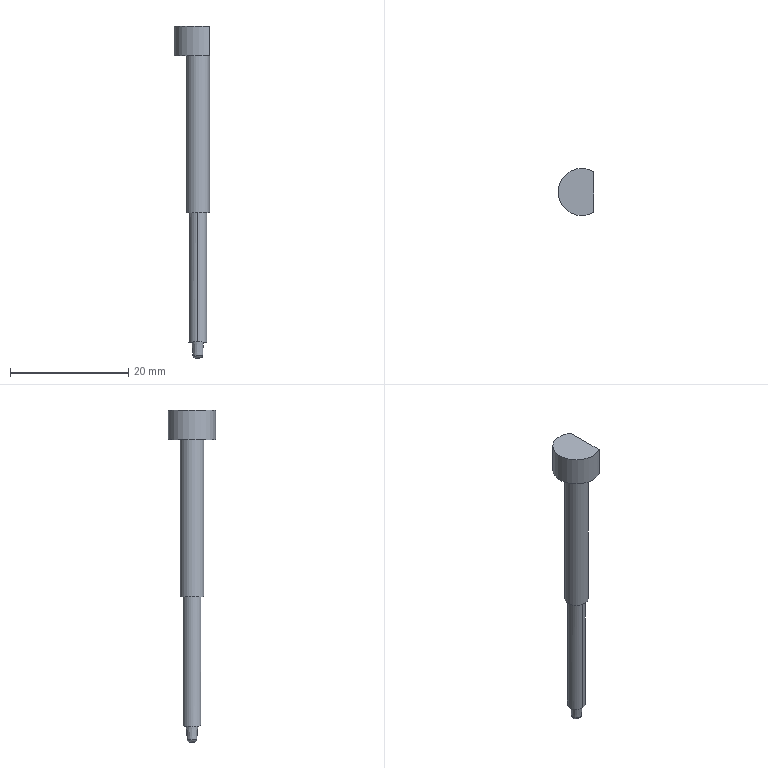Part | NX | features solid 2 | 1 solid | 12 faces | box 6 x 8 x 56.264 mm | volume 699.912 mm3 | plane 5 | cylinder 4 | cone 2 | torus 1 | commonest cylinder face diameters 3.015 x2 4 x1 8 x1
STEP:
#1=CARTESIAN_POINT('',(2.,-37.688,38.875));
#2=VERTEX_POINT('',#1);
#3=CARTESIAN_POINT('',(0.,-37.688,38.875));
#4=DIRECTION('',(0.,0.,1.));
#5=DIRECTION('',(1.,0.,0.));
#6=AXIS2_PLACEMENT_3D('',#3,#4,#5);
#7=CIRCLE('',#6,2.);
#8=EDGE_CURVE('',#2,#2,#7,.F.);
#9=ORIENTED_EDGE('',*,*,#8,.F.);
#10=EDGE_LOOP('',(#9));
#11=FACE_BOUND('',#10,.T.);
#12=CARTESIAN_POINT('',(2.,-37.688,65.5));
#13=VERTEX_POINT('',#12);
#14=CARTESIAN_POINT('',(0.,-37.688,65.5));
#15=DIRECTION('',(0.,0.,-1.));
#16=DIRECTION('',(-1.,0.,0.));
#17=AXIS2_PLACEMENT_3D('',#14,#15,#16);
#18=CIRCLE('',#17,2.);
#19=EDGE_CURVE('',#13,#13,#18,.F.);
#20=ORIENTED_EDGE('',*,*,#19,.F.);
#21=EDGE_LOOP('',(#20));
#22=FACE_BOUND('',#21,.T.);
#23=CARTESIAN_POINT('',(0.,-37.688,117.875));
#24=DIRECTION('',(0.,0.,-1.));
#25=DIRECTION('',(-1.,0.,0.));
#26=AXIS2_PLACEMENT_3D('',#23,#24,#25);
#27=CYLINDRICAL_SURFACE('',#26,2.);
#28=ADVANCED_FACE('',(#11,#22),#27,.T.);
#29=CARTESIAN_POINT('',(2.,-41.152,65.5));
#30=VERTEX_POINT('',#29);
#31=CARTESIAN_POINT('',(2.,-34.223,65.5));
#32=VERTEX_POINT('',#31);
#33=CARTESIAN_POINT('',(0.,-37.688,65.5));
#34=DIRECTION('',(0.,0.,-1.));
#35=DIRECTION('',(-1.,0.,0.));
#36=AXIS2_PLACEMENT_3D('',#33,#34,#35);
#37=CIRCLE('',#36,4.);
#38=EDGE_CURVE('',#30,#32,#37,.T.);
#39=ORIENTED_EDGE('',*,*,#38,.F.);
#40=CARTESIAN_POINT('',(2.,-41.152,70.5));
#41=VERTEX_POINT('',#40);
#42=CARTESIAN_POINT('',(2.,-41.152,66.5));
#43=DIRECTION('',(0.,0.,1.));
#44=VECTOR('',#43,1000.);
#45=LINE('',#42,#44);
#46=EDGE_CURVE('',#41,#30,#45,.F.);
#47=ORIENTED_EDGE('',*,*,#46,.F.);
#48=CARTESIAN_POINT('',(2.,-34.223,70.5));
#49=VERTEX_POINT('',#48);
#50=CARTESIAN_POINT('',(0.,-37.688,70.5));
#51=DIRECTION('',(0.,0.,1.));
#52=DIRECTION('',(1.,0.,0.));
#53=AXIS2_PLACEMENT_3D('',#50,#51,#52);
#54=CIRCLE('',#53,4.);
#55=EDGE_CURVE('',#41,#49,#54,.F.);
#56=ORIENTED_EDGE('',*,*,#55,.T.);
#57=CARTESIAN_POINT('',(2.,-34.223,66.5));
#58=DIRECTION('',(0.,0.,1.));
#59=VECTOR('',#58,1000.);
#60=LINE('',#57,#59);
#61=EDGE_CURVE('',#32,#49,#60,.T.);
#62=ORIENTED_EDGE('',*,*,#61,.F.);
#63=EDGE_LOOP('',(#39,#47,#56,#62));
#64=FACE_BOUND('',#63,.T.);
#65=CARTESIAN_POINT('',(0.,-37.688,66.5));
#66=DIRECTION('',(0.,0.,1.));
#67=DIRECTION('',(1.,0.,0.));
#68=AXIS2_PLACEMENT_3D('',#65,#66,#67);
#69=CYLINDRICAL_SURFACE('',#68,4.);
#70=ADVANCED_FACE('',(#64),#69,.T.);
#71=CARTESIAN_POINT('',(2.,37.688,65.5));
#72=DIRECTION('',(0.,-1.,0.));
#73=VECTOR('',#72,1000.);
#74=LINE('',#71,#73);
#75=EDGE_CURVE('',#13,#32,#74,.F.);
#76=ORIENTED_EDGE('',*,*,#75,.F.);
#77=ORIENTED_EDGE('',*,*,#19,.T.);
#78=CARTESIAN_POINT('',(2.,37.688,65.5));
#79=DIRECTION('',(0.,-1.,0.));
#80=VECTOR('',#79,1000.);
#81=LINE('',#78,#80);
#82=EDGE_CURVE('',#30,#13,#81,.F.);
#83=ORIENTED_EDGE('',*,*,#82,.F.);
#84=ORIENTED_EDGE('',*,*,#38,.T.);
#85=EDGE_LOOP('',(#76,#77,#83,#84));
#86=FACE_BOUND('',#85,.T.);
#87=CARTESIAN_POINT('',(0.,37.688,65.5));
#88=DIRECTION('',(0.,0.,-1.));
#89=DIRECTION('',(-1.,0.,0.));
#90=AXIS2_PLACEMENT_3D('',#87,#88,#89);
#91=PLANE('',#90);
#92=ADVANCED_FACE('',(#86),#91,.T.);
#93=CARTESIAN_POINT('',(2.,0.,70.5));
#94=DIRECTION('',(0.,1.,0.));
#95=VECTOR('',#94,1000.);
#96=LINE('',#93,#95);
#97=EDGE_CURVE('',#49,#41,#96,.F.);
#98=ORIENTED_EDGE('',*,*,#97,.F.);
#99=ORIENTED_EDGE('',*,*,#55,.F.);
#100=EDGE_LOOP('',(#98,#99));
#101=FACE_BOUND('',#100,.T.);
#102=CARTESIAN_POINT('',(0.,0.,70.5));
#103=DIRECTION('',(0.,0.,1.));
#104=DIRECTION('',(1.,0.,0.));
#105=AXIS2_PLACEMENT_3D('',#102,#103,#104);
#106=PLANE('',#105);
#107=ADVANCED_FACE('',(#101),#106,.T.);
#108=CARTESIAN_POINT('',(0.,-36.18,38.875));
#109=VERTEX_POINT('',#108);
#110=CARTESIAN_POINT('',(0.,-39.195,38.875));
#111=VERTEX_POINT('',#110);
#112=CARTESIAN_POINT('',(0.,-37.688,38.875));
#113=DIRECTION('',(0.,0.,1.));
#114=DIRECTION('',(0.,-1.,0.));
#115=AXIS2_PLACEMENT_3D('',#112,#113,#114);
#116=CIRCLE('',#115,1.508);
#117=EDGE_CURVE('',#109,#111,#116,.F.);
#118=ORIENTED_EDGE('',*,*,#117,.T.);
#119=CARTESIAN_POINT('',(0.,-39.195,16.996));
#120=VERTEX_POINT('',#119);
#121=CARTESIAN_POINT('',(0.,-39.195,38.875));
#122=DIRECTION('',(0.,0.,-1.));
#123=VECTOR('',#122,1000.);
#124=LINE('',#121,#123);
#125=EDGE_CURVE('',#120,#111,#124,.F.);
#126=ORIENTED_EDGE('',*,*,#125,.F.);
#127=CARTESIAN_POINT('',(0.,-36.18,16.969));
#128=VERTEX_POINT('',#127);
#129=CARTESIAN_POINT('',(0.,-39.195,16.996));
#130=CARTESIAN_POINT('',(0.3992,-39.195,16.996));
#131=CARTESIAN_POINT('',(1.178,-38.868,16.924));
#132=CARTESIAN_POINT('',(1.672,-37.691,16.809));
#133=CARTESIAN_POINT('',(1.18,-36.507,16.903));
#134=CARTESIAN_POINT('',(0.3992,-36.18,16.969));
#135=CARTESIAN_POINT('',(0.,-36.18,16.969));
#136=B_SPLINE_CURVE_WITH_KNOTS('',3,(#129,#130,#131,#132,#133,#134,#135),.UNSPECIFIED.,.F.,.F.,(4,1,1,1,4),(0.,0.00118,0.002361,0.003541,0.004722),.UNSPECIFIED.);
#137=EDGE_CURVE('',#120,#128,#136,.T.);
#138=ORIENTED_EDGE('',*,*,#137,.T.);
#139=CARTESIAN_POINT('',(0.,-36.18,16.969));
#140=DIRECTION('',(0.,0.,1.));
#141=VECTOR('',#140,1000.);
#142=LINE('',#139,#141);
#143=EDGE_CURVE('',#109,#128,#142,.F.);
#144=ORIENTED_EDGE('',*,*,#143,.F.);
#145=EDGE_LOOP('',(#118,#126,#138,#144));
#146=FACE_BOUND('',#145,.T.);
#147=CARTESIAN_POINT('',(0.,-37.688,38.875));
#148=DIRECTION('',(0.,0.,1.));
#149=DIRECTION('',(0.,1.,0.));
#150=AXIS2_PLACEMENT_3D('',#147,#148,#149);
#151=CYLINDRICAL_SURFACE('',#150,1.508);
#152=ADVANCED_FACE('',(#146),#151,.T.);
#153=CARTESIAN_POINT('',(0.,-37.688,38.875));
#154=DIRECTION('',(0.,0.,1.));
#155=DIRECTION('',(0.,1.,0.));
#156=AXIS2_PLACEMENT_3D('',#153,#154,#155);
#157=CIRCLE('',#156,1.508);
#158=EDGE_CURVE('',#111,#109,#157,.F.);
#159=ORIENTED_EDGE('',*,*,#158,.T.);
#160=ORIENTED_EDGE('',*,*,#143,.T.);
#161=CARTESIAN_POINT('',(0.,-36.18,16.969));
#162=CARTESIAN_POINT('',(-0.3992,-36.18,16.969));
#163=CARTESIAN_POINT('',(-1.179,-36.507,16.903));
#164=CARTESIAN_POINT('',(-1.672,-37.687,16.809));
#165=CARTESIAN_POINT('',(-1.179,-38.868,16.924));
#166=CARTESIAN_POINT('',(-0.3992,-39.195,16.996));
#167=CARTESIAN_POINT('',(0.,-39.195,16.996));
#168=B_SPLINE_CURVE_WITH_KNOTS('',3,(#161,#162,#163,#164,#165,#166,#167),.UNSPECIFIED.,.F.,.F.,(4,1,1,1,4),(0.,0.00118,0.002361,0.003541,0.004722),.UNSPECIFIED.);
#169=EDGE_CURVE('',#128,#120,#168,.T.);
#170=ORIENTED_EDGE('',*,*,#169,.T.);
#171=ORIENTED_EDGE('',*,*,#125,.T.);
#172=EDGE_LOOP('',(#159,#160,#170,#171));
#173=FACE_BOUND('',#172,.T.);
#174=CARTESIAN_POINT('',(0.,-37.688,38.875));
#175=DIRECTION('',(0.,0.,1.));
#176=DIRECTION('',(0.,1.,0.));
#177=AXIS2_PLACEMENT_3D('',#174,#175,#176);
#178=CYLINDRICAL_SURFACE('',#177,1.508);
#179=ADVANCED_FACE('',(#173),#178,.T.);
#180=ORIENTED_EDGE('',*,*,#8,.T.);
#181=EDGE_LOOP('',(#180));
#182=FACE_BOUND('',#181,.T.);
#183=ORIENTED_EDGE('',*,*,#158,.F.);
#184=ORIENTED_EDGE('',*,*,#117,.F.);
#185=EDGE_LOOP('',(#183,#184));
#186=FACE_BOUND('',#185,.T.);
#187=CARTESIAN_POINT('',(0.,-37.688,38.875));
#188=DIRECTION('',(0.,0.,1.));
#189=DIRECTION('',(0.,1.,0.));
#190=AXIS2_PLACEMENT_3D('',#187,#188,#189);
#191=PLANE('',#190);
#192=ADVANCED_FACE('',(#182,#186),#191,.F.);
#193=CARTESIAN_POINT('',(-0.3458,-37.688,14.236));
#194=VERTEX_POINT('',#193);
#195=CARTESIAN_POINT('',(0.,-37.688,14.236));
#196=DIRECTION('',(0.,0.,-1.));
#197=DIRECTION('',(-1.,0.,0.));
#198=AXIS2_PLACEMENT_3D('',#195,#196,#197);
#199=CIRCLE('',#198,0.3458);
#200=EDGE_CURVE('',#194,#194,#199,.T.);
#201=ORIENTED_EDGE('',*,*,#200,.T.);
#202=EDGE_LOOP('',(#201));
#203=FACE_BOUND('',#202,.T.);
#204=CARTESIAN_POINT('',(0.,-37.688,14.236));
#205=DIRECTION('',(0.,0.,-1.));
#206=DIRECTION('',(-1.,0.,0.));
#207=AXIS2_PLACEMENT_3D('',#204,#205,#206);
#208=PLANE('',#207);
#209=ADVANCED_FACE('',(#203),#208,.T.);
#210=CARTESIAN_POINT('',(-0.8451,-37.688,14.71));
#211=VERTEX_POINT('',#210);
#212=CARTESIAN_POINT('',(0.,-37.688,14.71));
#213=DIRECTION('',(0.,0.,-1.));
#214=DIRECTION('',(-1.,0.,0.));
#215=AXIS2_PLACEMENT_3D('',#212,#213,#214);
#216=CIRCLE('',#215,0.8451);
#217=EDGE_CURVE('',#211,#211,#216,.F.);
#218=ORIENTED_EDGE('',*,*,#217,.T.);
#219=EDGE_LOOP('',(#218));
#220=FACE_BOUND('',#219,.T.);
#221=CARTESIAN_POINT('',(0.8766,-37.292,16.933));
#222=VERTEX_POINT('',#221);
#223=CARTESIAN_POINT('',(0.3775,-36.688,16.977));
#224=CARTESIAN_POINT('',(0.9717,-37.25,16.923));
#225=CARTESIAN_POINT('',(0.9956,-38.066,16.926));
#226=CARTESIAN_POINT('',(0.4399,-38.661,16.991));
#227=CARTESIAN_POINT('',(-0.3781,-38.687,16.995));
#228=CARTESIAN_POINT('',(-0.9707,-38.127,16.931));
#229=CARTESIAN_POINT('',(-0.9966,-37.312,16.92));
#230=CARTESIAN_POINT('',(-0.4401,-36.714,16.974));
#231=CARTESIAN_POINT('',(0.3775,-36.688,16.977));
#232=CARTESIAN_POINT('',(0.9717,-37.25,16.923));
#233=CARTESIAN_POINT('',(0.9956,-38.066,16.926));
#234=B_SPLINE_CURVE_WITH_KNOTS('',3,(#223,#224,#225,#226,#227,#228,#229,#230,#231,#232,#233),.UNSPECIFIED.,.T.,.F.,(1,1,1,1,1,1,1,1,1,1,1,1,1,1,1),(-0.002259,-0.001506,-0.0007531,0.,0.0007531,0.001506,0.002259,0.003012,0.003765,0.004518,0.005272,0.006025,0.006778,0.007531,0.008284),.UNSPECIFIED.);
#235=EDGE_CURVE('',#222,#222,#234,.T.);
#236=ORIENTED_EDGE('',*,*,#235,.T.);
#237=EDGE_LOOP('',(#236));
#238=FACE_BOUND('',#237,.T.);
#239=CARTESIAN_POINT('',(0.,-37.688,14.236));
#240=DIRECTION('',(0.,0.,1.));
#241=DIRECTION('',(-1.,0.,0.));
#242=AXIS2_PLACEMENT_3D('',#239,#240,#241);
#243=CONICAL_SURFACE('',#242,0.8203,0.05236);
#244=ADVANCED_FACE('',(#220,#238),#243,.T.);
#245=ORIENTED_EDGE('',*,*,#235,.F.);
#246=EDGE_LOOP('',(#245));
#247=FACE_BOUND('',#246,.T.);
#248=ORIENTED_EDGE('',*,*,#137,.F.);
#249=ORIENTED_EDGE('',*,*,#169,.F.);
#250=EDGE_LOOP('',(#248,#249));
#251=FACE_BOUND('',#250,.T.);
#252=CARTESIAN_POINT('',(0.,-42.901,8.725));
#253=DIRECTION('',(0.,-1.,0.));
#254=DIRECTION('',(0.,0.,1.));
#255=AXIS2_PLACEMENT_3D('',#252,#253,#254);
#256=CONICAL_SURFACE('',#255,8.303,0.008727);
#257=ADVANCED_FACE('',(#247,#251),#256,.F.);
#258=ORIENTED_EDGE('',*,*,#82,.T.);
#259=ORIENTED_EDGE('',*,*,#75,.T.);
#260=ORIENTED_EDGE('',*,*,#61,.T.);
#261=ORIENTED_EDGE('',*,*,#97,.T.);
#262=ORIENTED_EDGE('',*,*,#46,.T.);
#263=EDGE_LOOP('',(#258,#259,#260,#261,#262));
#264=FACE_BOUND('',#263,.T.);
#265=CARTESIAN_POINT('',(2.,-37.688,65.5));
#266=DIRECTION('',(1.,0.,0.));
#267=DIRECTION('',(0.,0.,-1.));
#268=AXIS2_PLACEMENT_3D('',#265,#266,#267);
#269=PLANE('',#268);
#270=ADVANCED_FACE('',(#264),#269,.T.);
#271=ORIENTED_EDGE('',*,*,#200,.F.);
#272=EDGE_LOOP('',(#271));
#273=FACE_BOUND('',#272,.T.);
#274=ORIENTED_EDGE('',*,*,#217,.F.);
#275=EDGE_LOOP('',(#274));
#276=FACE_BOUND('',#275,.T.);
#277=CARTESIAN_POINT('',(0.,-37.688,14.736));
#278=DIRECTION('',(0.,0.,-1.));
#279=DIRECTION('',(-1.,0.,0.));
#280=AXIS2_PLACEMENT_3D('',#277,#278,#279);
#281=DEGENERATE_TOROIDAL_SURFACE('',#280,0.3458,0.5,.T.);
#282=ADVANCED_FACE('',(#273,#276),#281,.T.);
#283=CLOSED_SHELL('',(#28,#70,#92,#107,#152,#179,#192,#209,#244,#257,#270,#282));
#284=MANIFOLD_SOLID_BREP('',#283);
#285=(LENGTH_UNIT()NAMED_UNIT(*)SI_UNIT(.MILLI.,.METRE.));
#286=UNCERTAINTY_MEASURE_WITH_UNIT(LENGTH_MEASURE(0.0508),#285,'','');
#287=(NAMED_UNIT(*)PLANE_ANGLE_UNIT()SI_UNIT($,.RADIAN.));
#288=(NAMED_UNIT(*)SI_UNIT($,.STERADIAN.)SOLID_ANGLE_UNIT());
#289=(GEOMETRIC_REPRESENTATION_CONTEXT(3)GLOBAL_UNCERTAINTY_ASSIGNED_CONTEXT((#286))GLOBAL_UNIT_ASSIGNED_CONTEXT((#285,#287,#288))REPRESENTATION_CONTEXT('',''));
#290=ADVANCED_BREP_SHAPE_REPRESENTATION('',(#284),#289);